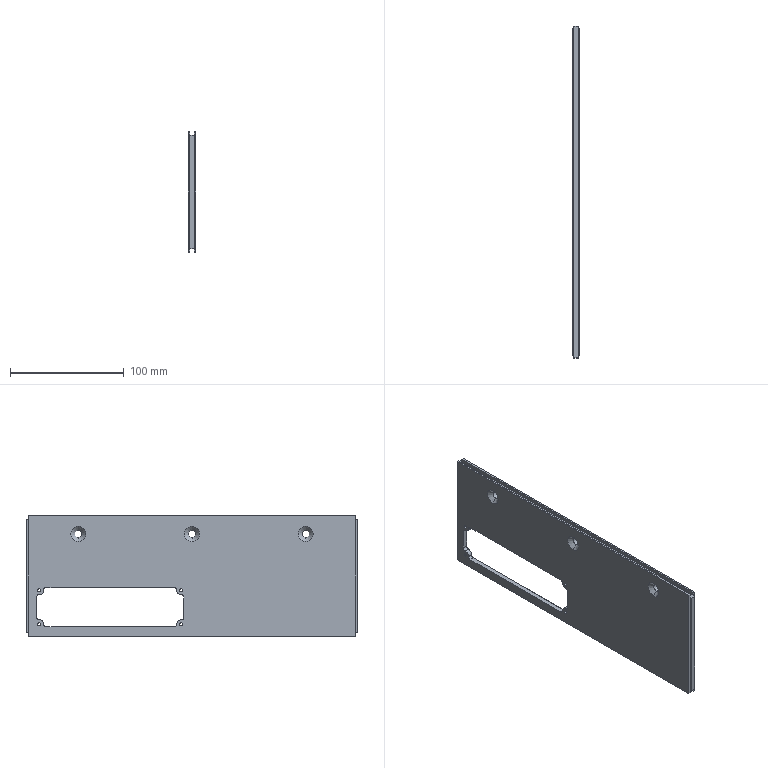Part | SolidWorks | features BaseBody 1 | 1 solid | 74 faces | box 7 x 292 x 106 mm | volume 173267 mm3 | plane 37 | cylinder 31 | cone 6 | commonest cylinder face diameters 2.6 x8 4 x8 6.4 x6 8 x5 10 x4